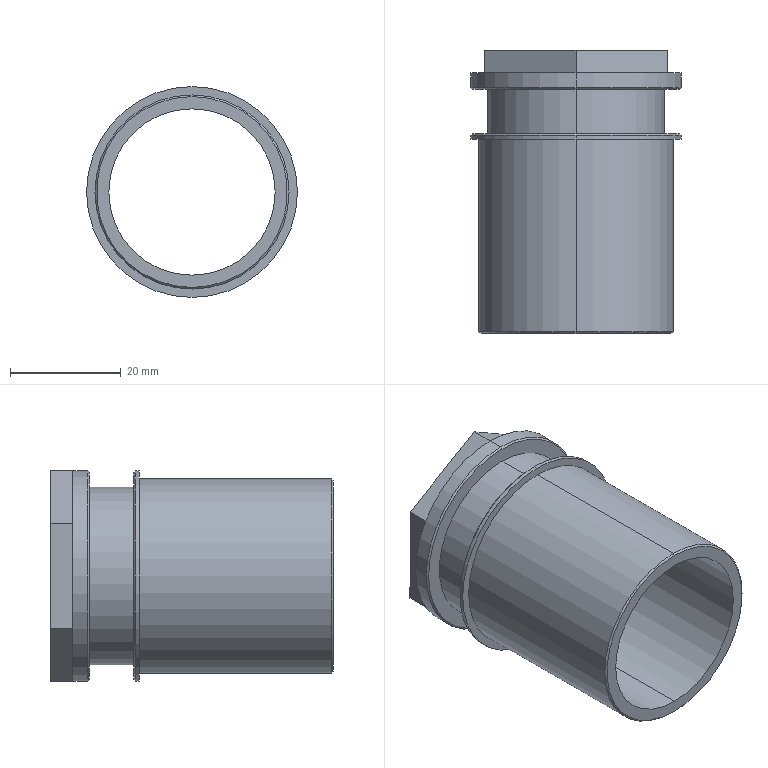Part | SolidWorks | features BaseBody 1 | 1 solid | 33 faces | box 38 x 51 x 38 mm | volume 12331 mm3 | plane 17 | cylinder 10 | cone 6 | commonest cylinder face diameters 38 x4 30 x2 32 x2 35 x2
STEP:
#1=CARTESIAN_POINT('',(0.,0.,-17.2));
#2=VERTEX_POINT('',#1);
#3=CARTESIAN_POINT('',(0.,0.,17.2));
#4=VERTEX_POINT('',#3);
#5=CARTESIAN_POINT('',(0.,0.,0.));
#6=DIRECTION('',(0.,-1.,0.));
#7=DIRECTION('',(0.,0.,1.));
#8=AXIS2_PLACEMENT_3D('',#5,#6,#7);
#9=CIRCLE('',#8,17.2);
#10=EDGE_CURVE('',#2,#4,#9,.T.);
#11=ORIENTED_EDGE('',*,*,#10,.F.);
#12=CARTESIAN_POINT('',(0.,0.3,-17.5));
#13=VERTEX_POINT('',#12);
#14=CARTESIAN_POINT('',(0.,0.3,-17.5));
#15=DIRECTION('',(0.,0.7071,-0.7071));
#16=VECTOR('',#15,1000.);
#17=LINE('',#14,#16);
#18=EDGE_CURVE('',#2,#13,#17,.T.);
#19=ORIENTED_EDGE('',*,*,#18,.T.);
#20=CARTESIAN_POINT('',(0.,0.3,17.5));
#21=VERTEX_POINT('',#20);
#22=CARTESIAN_POINT('',(0.,0.3,0.));
#23=DIRECTION('',(0.,1.,0.));
#24=DIRECTION('',(0.,0.,1.));
#25=AXIS2_PLACEMENT_3D('',#22,#23,#24);
#26=CIRCLE('',#25,17.5);
#27=EDGE_CURVE('',#21,#13,#26,.T.);
#28=ORIENTED_EDGE('',*,*,#27,.F.);
#29=CARTESIAN_POINT('',(0.,0.3,17.5));
#30=DIRECTION('',(0.,0.7071,0.7071));
#31=VECTOR('',#30,1000.);
#32=LINE('',#29,#31);
#33=EDGE_CURVE('',#4,#21,#32,.T.);
#34=ORIENTED_EDGE('',*,*,#33,.F.);
#35=EDGE_LOOP('',(#11,#19,#28,#34));
#36=FACE_OUTER_BOUND('',#35,.T.);
#37=CARTESIAN_POINT('',(0.,0.3,0.));
#38=DIRECTION('',(0.,1.,0.));
#39=DIRECTION('',(0.,0.,1.));
#40=AXIS2_PLACEMENT_3D('',#37,#38,#39);
#41=CONICAL_SURFACE('',#40,17.5,0.7854);
#42=ADVANCED_FACE('',(#36),#41,.T.);
#43=CARTESIAN_POINT('',(0.,44.,-18.7));
#44=VERTEX_POINT('',#43);
#45=CARTESIAN_POINT('',(0.,44.,18.7));
#46=VERTEX_POINT('',#45);
#47=CARTESIAN_POINT('',(0.,44.,0.));
#48=DIRECTION('',(0.,-1.,0.));
#49=DIRECTION('',(0.,0.,1.));
#50=AXIS2_PLACEMENT_3D('',#47,#48,#49);
#51=CIRCLE('',#50,18.7);
#52=EDGE_CURVE('',#44,#46,#51,.T.);
#53=ORIENTED_EDGE('',*,*,#52,.F.);
#54=CARTESIAN_POINT('',(0.,44.3,-19.));
#55=VERTEX_POINT('',#54);
#56=CARTESIAN_POINT('',(0.,44.3,-19.));
#57=DIRECTION('',(0.,0.7071,-0.7071));
#58=VECTOR('',#57,1000.);
#59=LINE('',#56,#58);
#60=EDGE_CURVE('',#44,#55,#59,.T.);
#61=ORIENTED_EDGE('',*,*,#60,.T.);
#62=CARTESIAN_POINT('',(0.,44.3,19.));
#63=VERTEX_POINT('',#62);
#64=CARTESIAN_POINT('',(0.,44.3,0.));
#65=DIRECTION('',(0.,1.,0.));
#66=DIRECTION('',(0.,0.,1.));
#67=AXIS2_PLACEMENT_3D('',#64,#65,#66);
#68=CIRCLE('',#67,19.);
#69=EDGE_CURVE('',#63,#55,#68,.T.);
#70=ORIENTED_EDGE('',*,*,#69,.F.);
#71=CARTESIAN_POINT('',(0.,44.3,19.));
#72=DIRECTION('',(0.,0.7071,0.7071));
#73=VECTOR('',#72,1000.);
#74=LINE('',#71,#73);
#75=EDGE_CURVE('',#46,#63,#74,.T.);
#76=ORIENTED_EDGE('',*,*,#75,.F.);
#77=EDGE_LOOP('',(#53,#61,#70,#76));
#78=FACE_OUTER_BOUND('',#77,.T.);
#79=CARTESIAN_POINT('',(0.,44.3,0.));
#80=DIRECTION('',(0.,1.,0.));
#81=DIRECTION('',(0.,0.,1.));
#82=AXIS2_PLACEMENT_3D('',#79,#80,#81);
#83=CONICAL_SURFACE('',#82,19.,0.7854);
#84=ADVANCED_FACE('',(#78),#83,.T.);
#85=CARTESIAN_POINT('',(0.,36.,18.7));
#86=VERTEX_POINT('',#85);
#87=CARTESIAN_POINT('',(0.,36.,-18.7));
#88=VERTEX_POINT('',#87);
#89=CARTESIAN_POINT('',(0.,36.,0.));
#90=DIRECTION('',(0.,1.,0.));
#91=DIRECTION('',(0.,0.,1.));
#92=AXIS2_PLACEMENT_3D('',#89,#90,#91);
#93=CIRCLE('',#92,18.7);
#94=EDGE_CURVE('',#86,#88,#93,.T.);
#95=ORIENTED_EDGE('',*,*,#94,.F.);
#96=CARTESIAN_POINT('',(0.,35.7,19.));
#97=VERTEX_POINT('',#96);
#98=CARTESIAN_POINT('',(0.,36.,18.7));
#99=DIRECTION('',(0.,-0.7071,0.7071));
#100=VECTOR('',#99,1000.);
#101=LINE('',#98,#100);
#102=EDGE_CURVE('',#86,#97,#101,.T.);
#103=ORIENTED_EDGE('',*,*,#102,.T.);
#104=CARTESIAN_POINT('',(0.,35.7,-19.));
#105=VERTEX_POINT('',#104);
#106=CARTESIAN_POINT('',(0.,35.7,0.));
#107=DIRECTION('',(0.,-1.,0.));
#108=DIRECTION('',(0.,0.,1.));
#109=AXIS2_PLACEMENT_3D('',#106,#107,#108);
#110=CIRCLE('',#109,19.);
#111=EDGE_CURVE('',#105,#97,#110,.T.);
#112=ORIENTED_EDGE('',*,*,#111,.F.);
#113=CARTESIAN_POINT('',(0.,36.,-18.7));
#114=DIRECTION('',(0.,-0.7071,-0.7071));
#115=VECTOR('',#114,1000.);
#116=LINE('',#113,#115);
#117=EDGE_CURVE('',#88,#105,#116,.T.);
#118=ORIENTED_EDGE('',*,*,#117,.F.);
#119=EDGE_LOOP('',(#95,#103,#112,#118));
#120=FACE_OUTER_BOUND('',#119,.T.);
#121=CARTESIAN_POINT('',(0.,36.,0.));
#122=DIRECTION('',(0.,-1.,0.));
#123=DIRECTION('',(0.,0.,-1.));
#124=AXIS2_PLACEMENT_3D('',#121,#122,#123);
#125=CONICAL_SURFACE('',#124,18.7,0.7854);
#126=ADVANCED_FACE('',(#120),#125,.T.);
#127=CARTESIAN_POINT('',(0.,0.,-15.));
#128=VERTEX_POINT('',#127);
#129=CARTESIAN_POINT('',(0.,0.,15.));
#130=VERTEX_POINT('',#129);
#131=CARTESIAN_POINT('',(0.,0.,0.));
#132=DIRECTION('',(0.,1.,0.));
#133=DIRECTION('',(0.,0.,1.));
#134=AXIS2_PLACEMENT_3D('',#131,#132,#133);
#135=CIRCLE('',#134,15.);
#136=EDGE_CURVE('',#128,#130,#135,.T.);
#137=ORIENTED_EDGE('',*,*,#136,.F.);
#138=CARTESIAN_POINT('',(0.,51.,-15.));
#139=VERTEX_POINT('',#138);
#140=CARTESIAN_POINT('',(0.,0.,-15.));
#141=DIRECTION('',(0.,1.,0.));
#142=VECTOR('',#141,1000.);
#143=LINE('',#140,#142);
#144=EDGE_CURVE('',#128,#139,#143,.T.);
#145=ORIENTED_EDGE('',*,*,#144,.T.);
#146=CARTESIAN_POINT('',(0.,51.,15.));
#147=VERTEX_POINT('',#146);
#148=CARTESIAN_POINT('',(0.,51.,0.));
#149=DIRECTION('',(0.,1.,0.));
#150=DIRECTION('',(0.,0.,1.));
#151=AXIS2_PLACEMENT_3D('',#148,#149,#150);
#152=CIRCLE('',#151,15.);
#153=EDGE_CURVE('',#139,#147,#152,.T.);
#154=ORIENTED_EDGE('',*,*,#153,.T.);
#155=CARTESIAN_POINT('',(0.,0.,15.));
#156=DIRECTION('',(0.,1.,0.));
#157=VECTOR('',#156,1000.);
#158=LINE('',#155,#157);
#159=EDGE_CURVE('',#130,#147,#158,.T.);
#160=ORIENTED_EDGE('',*,*,#159,.F.);
#161=EDGE_LOOP('',(#137,#145,#154,#160));
#162=FACE_OUTER_BOUND('',#161,.T.);
#163=CARTESIAN_POINT('',(0.,0.,0.));
#164=DIRECTION('',(0.,1.,0.));
#165=DIRECTION('',(0.,0.,1.));
#166=AXIS2_PLACEMENT_3D('',#163,#164,#165);
#167=CYLINDRICAL_SURFACE('',#166,15.);
#168=ADVANCED_FACE('',(#162),#167,.F.);
#169=CARTESIAN_POINT('',(0.,35.,19.));
#170=VERTEX_POINT('',#169);
#171=CARTESIAN_POINT('',(0.,35.,-19.));
#172=VERTEX_POINT('',#171);
#173=CARTESIAN_POINT('',(0.,35.,0.));
#174=DIRECTION('',(0.,1.,0.));
#175=DIRECTION('',(0.,0.,1.));
#176=AXIS2_PLACEMENT_3D('',#173,#174,#175);
#177=CIRCLE('',#176,19.);
#178=EDGE_CURVE('',#170,#172,#177,.T.);
#179=ORIENTED_EDGE('',*,*,#178,.T.);
#180=CARTESIAN_POINT('',(0.,35.,-19.));
#181=DIRECTION('',(0.,1.,0.));
#182=VECTOR('',#181,1000.);
#183=LINE('',#180,#182);
#184=EDGE_CURVE('',#172,#105,#183,.T.);
#185=ORIENTED_EDGE('',*,*,#184,.T.);
#186=ORIENTED_EDGE('',*,*,#111,.T.);
#187=CARTESIAN_POINT('',(0.,35.,19.));
#188=DIRECTION('',(0.,1.,0.));
#189=VECTOR('',#188,1000.);
#190=LINE('',#187,#189);
#191=EDGE_CURVE('',#170,#97,#190,.T.);
#192=ORIENTED_EDGE('',*,*,#191,.F.);
#193=EDGE_LOOP('',(#179,#185,#186,#192));
#194=FACE_OUTER_BOUND('',#193,.T.);
#195=CARTESIAN_POINT('',(0.,35.,0.));
#196=DIRECTION('',(0.,1.,0.));
#197=DIRECTION('',(0.,0.,1.));
#198=AXIS2_PLACEMENT_3D('',#195,#196,#197);
#199=CYLINDRICAL_SURFACE('',#198,19.);
#200=ADVANCED_FACE('',(#194),#199,.T.);
#201=CARTESIAN_POINT('',(0.,35.,17.5));
#202=VERTEX_POINT('',#201);
#203=CARTESIAN_POINT('',(0.,35.,-17.5));
#204=VERTEX_POINT('',#203);
#205=CARTESIAN_POINT('',(0.,35.,0.));
#206=DIRECTION('',(0.,1.,0.));
#207=DIRECTION('',(0.,0.,1.));
#208=AXIS2_PLACEMENT_3D('',#205,#206,#207);
#209=CIRCLE('',#208,17.5);
#210=EDGE_CURVE('',#202,#204,#209,.T.);
#211=ORIENTED_EDGE('',*,*,#210,.F.);
#212=CARTESIAN_POINT('',(0.,36.,17.5));
#213=DIRECTION('',(0.,-1.,0.));
#214=VECTOR('',#213,1000.);
#215=LINE('',#212,#214);
#216=EDGE_CURVE('',#202,#21,#215,.T.);
#217=ORIENTED_EDGE('',*,*,#216,.T.);
#218=ORIENTED_EDGE('',*,*,#27,.T.);
#219=CARTESIAN_POINT('',(0.,36.,-17.5));
#220=DIRECTION('',(0.,-1.,0.));
#221=VECTOR('',#220,1000.);
#222=LINE('',#219,#221);
#223=EDGE_CURVE('',#204,#13,#222,.T.);
#224=ORIENTED_EDGE('',*,*,#223,.F.);
#225=EDGE_LOOP('',(#211,#217,#218,#224));
#226=FACE_OUTER_BOUND('',#225,.T.);
#227=CARTESIAN_POINT('',(0.,36.,0.));
#228=DIRECTION('',(0.,-1.,0.));
#229=DIRECTION('',(0.,0.,-1.));
#230=AXIS2_PLACEMENT_3D('',#227,#228,#229);
#231=CYLINDRICAL_SURFACE('',#230,17.5);
#232=ADVANCED_FACE('',(#226),#231,.T.);
#233=CARTESIAN_POINT('',(0.,44.,16.));
#234=VERTEX_POINT('',#233);
#235=CARTESIAN_POINT('',(0.,44.,-16.));
#236=VERTEX_POINT('',#235);
#237=CARTESIAN_POINT('',(0.,44.,0.));
#238=DIRECTION('',(0.,1.,0.));
#239=DIRECTION('',(0.,0.,1.));
#240=AXIS2_PLACEMENT_3D('',#237,#238,#239);
#241=CIRCLE('',#240,16.);
#242=EDGE_CURVE('',#234,#236,#241,.T.);
#243=ORIENTED_EDGE('',*,*,#242,.F.);
#244=CARTESIAN_POINT('',(0.,36.,16.));
#245=VERTEX_POINT('',#244);
#246=CARTESIAN_POINT('',(0.,51.,16.));
#247=DIRECTION('',(0.,-1.,0.));
#248=VECTOR('',#247,1000.);
#249=LINE('',#246,#248);
#250=EDGE_CURVE('',#234,#245,#249,.T.);
#251=ORIENTED_EDGE('',*,*,#250,.T.);
#252=CARTESIAN_POINT('',(0.,36.,-16.));
#253=VERTEX_POINT('',#252);
#254=CARTESIAN_POINT('',(0.,36.,0.));
#255=DIRECTION('',(0.,1.,0.));
#256=DIRECTION('',(0.,0.,1.));
#257=AXIS2_PLACEMENT_3D('',#254,#255,#256);
#258=CIRCLE('',#257,16.);
#259=EDGE_CURVE('',#245,#253,#258,.T.);
#260=ORIENTED_EDGE('',*,*,#259,.T.);
#261=CARTESIAN_POINT('',(0.,51.,-16.));
#262=DIRECTION('',(0.,-1.,0.));
#263=VECTOR('',#262,1000.);
#264=LINE('',#261,#263);
#265=EDGE_CURVE('',#236,#253,#264,.T.);
#266=ORIENTED_EDGE('',*,*,#265,.F.);
#267=EDGE_LOOP('',(#243,#251,#260,#266));
#268=FACE_OUTER_BOUND('',#267,.T.);
#269=CARTESIAN_POINT('',(0.,51.,0.));
#270=DIRECTION('',(0.,-1.,0.));
#271=DIRECTION('',(0.,0.,-1.));
#272=AXIS2_PLACEMENT_3D('',#269,#270,#271);
#273=CYLINDRICAL_SURFACE('',#272,16.);
#274=ADVANCED_FACE('',(#268),#273,.T.);
#275=ORIENTED_EDGE('',*,*,#69,.T.);
#276=CARTESIAN_POINT('',(0.,47.,-19.));
#277=VERTEX_POINT('',#276);
#278=CARTESIAN_POINT('',(0.,44.,-19.));
#279=DIRECTION('',(0.,1.,0.));
#280=VECTOR('',#279,1000.);
#281=LINE('',#278,#280);
#282=EDGE_CURVE('',#55,#277,#281,.T.);
#283=ORIENTED_EDGE('',*,*,#282,.T.);
#284=CARTESIAN_POINT('',(16.454,47.,-9.5));
#285=VERTEX_POINT('',#284);
#286=CARTESIAN_POINT('',(0.,47.,0.));
#287=DIRECTION('',(0.,-1.,0.));
#288=DIRECTION('',(0.,0.,1.));
#289=AXIS2_PLACEMENT_3D('',#286,#287,#288);
#290=CIRCLE('',#289,19.);
#291=EDGE_CURVE('',#277,#285,#290,.T.);
#292=ORIENTED_EDGE('',*,*,#291,.T.);
#293=CARTESIAN_POINT('',(16.454,47.,9.5));
#294=VERTEX_POINT('',#293);
#295=CARTESIAN_POINT('',(0.,47.,0.));
#296=DIRECTION('',(0.,-1.,0.));
#297=DIRECTION('',(0.,0.,1.));
#298=AXIS2_PLACEMENT_3D('',#295,#296,#297);
#299=CIRCLE('',#298,19.);
#300=EDGE_CURVE('',#285,#294,#299,.T.);
#301=ORIENTED_EDGE('',*,*,#300,.T.);
#302=CARTESIAN_POINT('',(0.,47.,19.));
#303=VERTEX_POINT('',#302);
#304=CARTESIAN_POINT('',(0.,47.,0.));
#305=DIRECTION('',(0.,-1.,0.));
#306=DIRECTION('',(0.,0.,1.));
#307=AXIS2_PLACEMENT_3D('',#304,#305,#306);
#308=CIRCLE('',#307,19.);
#309=EDGE_CURVE('',#294,#303,#308,.T.);
#310=ORIENTED_EDGE('',*,*,#309,.T.);
#311=CARTESIAN_POINT('',(0.,44.,19.));
#312=DIRECTION('',(0.,1.,0.));
#313=VECTOR('',#312,1000.);
#314=LINE('',#311,#313);
#315=EDGE_CURVE('',#63,#303,#314,.T.);
#316=ORIENTED_EDGE('',*,*,#315,.F.);
#317=EDGE_LOOP('',(#275,#283,#292,#301,#310,#316));
#318=FACE_OUTER_BOUND('',#317,.T.);
#319=CARTESIAN_POINT('',(0.,44.,0.));
#320=DIRECTION('',(0.,1.,0.));
#321=DIRECTION('',(0.,0.,1.));
#322=AXIS2_PLACEMENT_3D('',#319,#320,#321);
#323=CYLINDRICAL_SURFACE('',#322,19.);
#324=ADVANCED_FACE('',(#318),#323,.T.);
#325=CARTESIAN_POINT('',(0.,51.,-19.));
#326=VERTEX_POINT('',#325);
#327=CARTESIAN_POINT('',(-16.454,51.,-9.5));
#328=VERTEX_POINT('',#327);
#329=CARTESIAN_POINT('',(0.,51.,-19.));
#330=DIRECTION('',(-0.866,0.,0.5));
#331=VECTOR('',#330,1000.);
#332=LINE('',#329,#331);
#333=EDGE_CURVE('',#326,#328,#332,.T.);
#334=ORIENTED_EDGE('',*,*,#333,.F.);
#335=CARTESIAN_POINT('',(0.,47.,-19.));
#336=DIRECTION('',(0.,1.,0.));
#337=VECTOR('',#336,1000.);
#338=LINE('',#335,#337);
#339=EDGE_CURVE('',#277,#326,#338,.T.);
#340=ORIENTED_EDGE('',*,*,#339,.F.);
#341=CARTESIAN_POINT('',(-16.454,47.,-9.5));
#342=VERTEX_POINT('',#341);
#343=CARTESIAN_POINT('',(0.,47.,-19.));
#344=DIRECTION('',(-0.866,0.,0.5));
#345=VECTOR('',#344,1000.);
#346=LINE('',#343,#345);
#347=EDGE_CURVE('',#277,#342,#346,.T.);
#348=ORIENTED_EDGE('',*,*,#347,.T.);
#349=CARTESIAN_POINT('',(-16.454,47.,-9.5));
#350=DIRECTION('',(0.,1.,0.));
#351=VECTOR('',#350,1000.);
#352=LINE('',#349,#351);
#353=EDGE_CURVE('',#342,#328,#352,.T.);
#354=ORIENTED_EDGE('',*,*,#353,.T.);
#355=EDGE_LOOP('',(#334,#340,#348,#354));
#356=FACE_OUTER_BOUND('',#355,.T.);
#357=CARTESIAN_POINT('',(0.,47.,-19.));
#358=DIRECTION('',(-0.5,0.,-0.866));
#359=DIRECTION('',(-0.866,0.,0.5));
#360=AXIS2_PLACEMENT_3D('',#357,#358,#359);
#361=PLANE('',#360);
#362=ADVANCED_FACE('',(#356),#361,.T.);
#363=CARTESIAN_POINT('',(-16.454,51.,9.5));
#364=VERTEX_POINT('',#363);
#365=CARTESIAN_POINT('',(-16.454,51.,-9.5));
#366=DIRECTION('',(0.,0.,1.));
#367=VECTOR('',#366,1000.);
#368=LINE('',#365,#367);
#369=EDGE_CURVE('',#328,#364,#368,.T.);
#370=ORIENTED_EDGE('',*,*,#369,.F.);
#371=ORIENTED_EDGE('',*,*,#353,.F.);
#372=CARTESIAN_POINT('',(-16.454,47.,9.5));
#373=VERTEX_POINT('',#372);
#374=CARTESIAN_POINT('',(-16.454,47.,-9.5));
#375=DIRECTION('',(0.,0.,1.));
#376=VECTOR('',#375,1000.);
#377=LINE('',#374,#376);
#378=EDGE_CURVE('',#342,#373,#377,.T.);
#379=ORIENTED_EDGE('',*,*,#378,.T.);
#380=CARTESIAN_POINT('',(-16.454,47.,9.5));
#381=DIRECTION('',(0.,1.,0.));
#382=VECTOR('',#381,1000.);
#383=LINE('',#380,#382);
#384=EDGE_CURVE('',#373,#364,#383,.T.);
#385=ORIENTED_EDGE('',*,*,#384,.T.);
#386=EDGE_LOOP('',(#370,#371,#379,#385));
#387=FACE_OUTER_BOUND('',#386,.T.);
#388=CARTESIAN_POINT('',(-16.454,47.,-9.5));
#389=DIRECTION('',(-1.,0.,0.));
#390=DIRECTION('',(0.,1.,0.));
#391=AXIS2_PLACEMENT_3D('',#388,#389,#390);
#392=PLANE('',#391);
#393=ADVANCED_FACE('',(#387),#392,.T.);
#394=CARTESIAN_POINT('',(0.,51.,19.));
#395=VERTEX_POINT('',#394);
#396=CARTESIAN_POINT('',(-16.454,51.,9.5));
#397=DIRECTION('',(0.866,0.,0.5));
#398=VECTOR('',#397,1000.);
#399=LINE('',#396,#398);
#400=EDGE_CURVE('',#364,#395,#399,.T.);
#401=ORIENTED_EDGE('',*,*,#400,.F.);
#402=ORIENTED_EDGE('',*,*,#384,.F.);
#403=CARTESIAN_POINT('',(-16.454,47.,9.5));
#404=DIRECTION('',(0.866,0.,0.5));
#405=VECTOR('',#404,1000.);
#406=LINE('',#403,#405);
#407=EDGE_CURVE('',#373,#303,#406,.T.);
#408=ORIENTED_EDGE('',*,*,#407,.T.);
#409=CARTESIAN_POINT('',(0.,47.,19.));
#410=DIRECTION('',(0.,1.,0.));
#411=VECTOR('',#410,1000.);
#412=LINE('',#409,#411);
#413=EDGE_CURVE('',#303,#395,#412,.T.);
#414=ORIENTED_EDGE('',*,*,#413,.T.);
#415=EDGE_LOOP('',(#401,#402,#408,#414));
#416=FACE_OUTER_BOUND('',#415,.T.);
#417=CARTESIAN_POINT('',(-16.454,47.,9.5));
#418=DIRECTION('',(-0.5,0.,0.866));
#419=DIRECTION('',(0.,1.,0.));
#420=AXIS2_PLACEMENT_3D('',#417,#418,#419);
#421=PLANE('',#420);
#422=ADVANCED_FACE('',(#416),#421,.T.);
#423=CARTESIAN_POINT('',(16.454,51.,9.5));
#424=VERTEX_POINT('',#423);
#425=CARTESIAN_POINT('',(0.,51.,19.));
#426=DIRECTION('',(0.866,0.,-0.5));
#427=VECTOR('',#426,1000.);
#428=LINE('',#425,#427);
#429=EDGE_CURVE('',#395,#424,#428,.T.);
#430=ORIENTED_EDGE('',*,*,#429,.F.);
#431=ORIENTED_EDGE('',*,*,#413,.F.);
#432=CARTESIAN_POINT('',(0.,47.,19.));
#433=DIRECTION('',(0.866,0.,-0.5));
#434=VECTOR('',#433,1000.);
#435=LINE('',#432,#434);
#436=EDGE_CURVE('',#303,#294,#435,.T.);
#437=ORIENTED_EDGE('',*,*,#436,.T.);
#438=CARTESIAN_POINT('',(16.454,47.,9.5));
#439=DIRECTION('',(0.,1.,0.));
#440=VECTOR('',#439,1000.);
#441=LINE('',#438,#440);
#442=EDGE_CURVE('',#294,#424,#441,.T.);
#443=ORIENTED_EDGE('',*,*,#442,.T.);
#444=EDGE_LOOP('',(#430,#431,#437,#443));
#445=FACE_OUTER_BOUND('',#444,.T.);
#446=CARTESIAN_POINT('',(0.,47.,19.));
#447=DIRECTION('',(0.5,0.,0.866));
#448=DIRECTION('',(0.,-1.,0.));
#449=AXIS2_PLACEMENT_3D('',#446,#447,#448);
#450=PLANE('',#449);
#451=ADVANCED_FACE('',(#445),#450,.T.);
#452=CARTESIAN_POINT('',(16.454,51.,-9.5));
#453=VERTEX_POINT('',#452);
#454=CARTESIAN_POINT('',(16.454,51.,9.5));
#455=DIRECTION('',(0.,0.,-1.));
#456=VECTOR('',#455,1000.);
#457=LINE('',#454,#456);
#458=EDGE_CURVE('',#424,#453,#457,.T.);
#459=ORIENTED_EDGE('',*,*,#458,.F.);
#460=ORIENTED_EDGE('',*,*,#442,.F.);
#461=CARTESIAN_POINT('',(16.454,47.,9.5));
#462=DIRECTION('',(0.,0.,-1.));
#463=VECTOR('',#462,1000.);
#464=LINE('',#461,#463);
#465=EDGE_CURVE('',#294,#285,#464,.T.);
#466=ORIENTED_EDGE('',*,*,#465,.T.);
#467=CARTESIAN_POINT('',(16.454,47.,-9.5));
#468=DIRECTION('',(0.,1.,0.));
#469=VECTOR('',#468,1000.);
#470=LINE('',#467,#469);
#471=EDGE_CURVE('',#285,#453,#470,.T.);
#472=ORIENTED_EDGE('',*,*,#471,.T.);
#473=EDGE_LOOP('',(#459,#460,#466,#472));
#474=FACE_OUTER_BOUND('',#473,.T.);
#475=CARTESIAN_POINT('',(16.454,47.,9.5));
#476=DIRECTION('',(1.,0.,0.));
#477=DIRECTION('',(0.,1.,0.));
#478=AXIS2_PLACEMENT_3D('',#475,#476,#477);
#479=PLANE('',#478);
#480=ADVANCED_FACE('',(#474),#479,.T.);
#481=CARTESIAN_POINT('',(16.454,51.,-9.5));
#482=DIRECTION('',(-0.866,0.,-0.5));
#483=VECTOR('',#482,1000.);
#484=LINE('',#481,#483);
#485=EDGE_CURVE('',#453,#326,#484,.T.);
#486=ORIENTED_EDGE('',*,*,#485,.F.);
#487=ORIENTED_EDGE('',*,*,#471,.F.);
#488=CARTESIAN_POINT('',(16.454,47.,-9.5));
#489=DIRECTION('',(-0.866,0.,-0.5));
#490=VECTOR('',#489,1000.);
#491=LINE('',#488,#490);
#492=EDGE_CURVE('',#285,#277,#491,.T.);
#493=ORIENTED_EDGE('',*,*,#492,.T.);
#494=ORIENTED_EDGE('',*,*,#339,.T.);
#495=EDGE_LOOP('',(#486,#487,#493,#494));
#496=FACE_OUTER_BOUND('',#495,.T.);
#497=CARTESIAN_POINT('',(16.454,47.,-9.5));
#498=DIRECTION('',(0.5,0.,-0.866));
#499=DIRECTION('',(0.,-1.,0.));
#500=AXIS2_PLACEMENT_3D('',#497,#498,#499);
#501=PLANE('',#500);
#502=ADVANCED_FACE('',(#496),#501,.T.);
#503=ORIENTED_EDGE('',*,*,#436,.F.);
#504=ORIENTED_EDGE('',*,*,#309,.F.);
#505=EDGE_LOOP('',(#503,#504));
#506=FACE_OUTER_BOUND('',#505,.T.);
#507=CARTESIAN_POINT('',(0.,47.,0.));
#508=DIRECTION('',(0.,1.,0.));
#509=DIRECTION('',(1.,0.,0.));
#510=AXIS2_PLACEMENT_3D('',#507,#508,#509);
#511=PLANE('',#510);
#512=ADVANCED_FACE('',(#506),#511,.T.);
#513=ORIENTED_EDGE('',*,*,#465,.F.);
#514=ORIENTED_EDGE('',*,*,#300,.F.);
#515=EDGE_LOOP('',(#513,#514));
#516=FACE_OUTER_BOUND('',#515,.T.);
#517=CARTESIAN_POINT('',(0.,47.,0.));
#518=DIRECTION('',(0.,1.,0.));
#519=DIRECTION('',(1.,0.,0.));
#520=AXIS2_PLACEMENT_3D('',#517,#518,#519);
#521=PLANE('',#520);
#522=ADVANCED_FACE('',(#516),#521,.T.);
#523=ORIENTED_EDGE('',*,*,#492,.F.);
#524=ORIENTED_EDGE('',*,*,#291,.F.);
#525=EDGE_LOOP('',(#523,#524));
#526=FACE_OUTER_BOUND('',#525,.T.);
#527=CARTESIAN_POINT('',(0.,47.,0.));
#528=DIRECTION('',(0.,1.,0.));
#529=DIRECTION('',(1.,0.,0.));
#530=AXIS2_PLACEMENT_3D('',#527,#528,#529);
#531=PLANE('',#530);
#532=ADVANCED_FACE('',(#526),#531,.T.);
#533=ORIENTED_EDGE('',*,*,#347,.F.);
#534=CARTESIAN_POINT('',(0.,47.,0.));
#535=DIRECTION('',(0.,-1.,0.));
#536=DIRECTION('',(0.,0.,1.));
#537=AXIS2_PLACEMENT_3D('',#534,#535,#536);
#538=CIRCLE('',#537,19.);
#539=EDGE_CURVE('',#342,#277,#538,.T.);
#540=ORIENTED_EDGE('',*,*,#539,.F.);
#541=EDGE_LOOP('',(#533,#540));
#542=FACE_OUTER_BOUND('',#541,.T.);
#543=CARTESIAN_POINT('',(0.,47.,0.));
#544=DIRECTION('',(0.,1.,0.));
#545=DIRECTION('',(1.,0.,0.));
#546=AXIS2_PLACEMENT_3D('',#543,#544,#545);
#547=PLANE('',#546);
#548=ADVANCED_FACE('',(#542),#547,.T.);
#549=ORIENTED_EDGE('',*,*,#378,.F.);
#550=CARTESIAN_POINT('',(0.,47.,0.));
#551=DIRECTION('',(0.,-1.,0.));
#552=DIRECTION('',(0.,0.,1.));
#553=AXIS2_PLACEMENT_3D('',#550,#551,#552);
#554=CIRCLE('',#553,19.);
#555=EDGE_CURVE('',#373,#342,#554,.T.);
#556=ORIENTED_EDGE('',*,*,#555,.F.);
#557=EDGE_LOOP('',(#549,#556));
#558=FACE_OUTER_BOUND('',#557,.T.);
#559=CARTESIAN_POINT('',(0.,47.,0.));
#560=DIRECTION('',(0.,1.,0.));
#561=DIRECTION('',(1.,0.,0.));
#562=AXIS2_PLACEMENT_3D('',#559,#560,#561);
#563=PLANE('',#562);
#564=ADVANCED_FACE('',(#558),#563,.T.);
#565=ORIENTED_EDGE('',*,*,#407,.F.);
#566=CARTESIAN_POINT('',(0.,47.,0.));
#567=DIRECTION('',(0.,-1.,0.));
#568=DIRECTION('',(0.,0.,1.));
#569=AXIS2_PLACEMENT_3D('',#566,#567,#568);
#570=CIRCLE('',#569,19.);
#571=EDGE_CURVE('',#303,#373,#570,.T.);
#572=ORIENTED_EDGE('',*,*,#571,.F.);
#573=EDGE_LOOP('',(#565,#572));
#574=FACE_OUTER_BOUND('',#573,.T.);
#575=CARTESIAN_POINT('',(0.,47.,0.));
#576=DIRECTION('',(0.,1.,0.));
#577=DIRECTION('',(1.,0.,0.));
#578=AXIS2_PLACEMENT_3D('',#575,#576,#577);
#579=PLANE('',#578);
#580=ADVANCED_FACE('',(#574),#579,.T.);
#581=CARTESIAN_POINT('',(0.,44.,0.));
#582=DIRECTION('',(0.,1.,0.));
#583=DIRECTION('',(0.,0.,1.));
#584=AXIS2_PLACEMENT_3D('',#581,#582,#583);
#585=CIRCLE('',#584,16.);
#586=EDGE_CURVE('',#236,#234,#585,.T.);
#587=ORIENTED_EDGE('',*,*,#586,.T.);
#588=ORIENTED_EDGE('',*,*,#242,.T.);
#589=EDGE_LOOP('',(#587,#588));
#590=FACE_BOUND('',#589,.T.);
#591=CARTESIAN_POINT('',(0.,44.,0.));
#592=DIRECTION('',(0.,-1.,0.));
#593=DIRECTION('',(0.,0.,1.));
#594=AXIS2_PLACEMENT_3D('',#591,#592,#593);
#595=CIRCLE('',#594,18.7);
#596=EDGE_CURVE('',#46,#44,#595,.T.);
#597=ORIENTED_EDGE('',*,*,#596,.T.);
#598=ORIENTED_EDGE('',*,*,#52,.T.);
#599=EDGE_LOOP('',(#597,#598));
#600=FACE_OUTER_BOUND('',#599,.T.);
#601=CARTESIAN_POINT('',(0.,44.,0.));
#602=DIRECTION('',(0.,1.,0.));
#603=DIRECTION('',(1.,0.,0.));
#604=AXIS2_PLACEMENT_3D('',#601,#602,#603);
#605=PLANE('',#604);
#606=ADVANCED_FACE('',(#590,#600),#605,.F.);
#607=CARTESIAN_POINT('',(0.,36.,0.));
#608=DIRECTION('',(0.,1.,0.));
#609=DIRECTION('',(0.,0.,1.));
#610=AXIS2_PLACEMENT_3D('',#607,#608,#609);
#611=CIRCLE('',#610,16.);
#612=EDGE_CURVE('',#253,#245,#611,.T.);
#613=ORIENTED_EDGE('',*,*,#612,.F.);
#614=ORIENTED_EDGE('',*,*,#259,.F.);
#615=EDGE_LOOP('',(#613,#614));
#616=FACE_BOUND('',#615,.T.);
#617=CARTESIAN_POINT('',(0.,36.,0.));
#618=DIRECTION('',(0.,1.,0.));
#619=DIRECTION('',(0.,0.,1.));
#620=AXIS2_PLACEMENT_3D('',#617,#618,#619);
#621=CIRCLE('',#620,18.7);
#622=EDGE_CURVE('',#88,#86,#621,.T.);
#623=ORIENTED_EDGE('',*,*,#622,.T.);
#624=ORIENTED_EDGE('',*,*,#94,.T.);
#625=EDGE_LOOP('',(#623,#624));
#626=FACE_OUTER_BOUND('',#625,.T.);
#627=CARTESIAN_POINT('',(0.,36.,0.));
#628=DIRECTION('',(0.,1.,0.));
#629=DIRECTION('',(1.,0.,0.));
#630=AXIS2_PLACEMENT_3D('',#627,#628,#629);
#631=PLANE('',#630);
#632=ADVANCED_FACE('',(#616,#626),#631,.T.);
#633=CARTESIAN_POINT('',(0.,35.,0.));
#634=DIRECTION('',(0.,1.,0.));
#635=DIRECTION('',(0.,0.,1.));
#636=AXIS2_PLACEMENT_3D('',#633,#634,#635);
#637=CIRCLE('',#636,17.5);
#638=EDGE_CURVE('',#204,#202,#637,.T.);
#639=ORIENTED_EDGE('',*,*,#638,.T.);
#640=ORIENTED_EDGE('',*,*,#210,.T.);
#641=EDGE_LOOP('',(#639,#640));
#642=FACE_BOUND('',#641,.T.);
#643=ORIENTED_EDGE('',*,*,#178,.F.);
#644=CARTESIAN_POINT('',(0.,35.,0.));
#645=DIRECTION('',(0.,1.,0.));
#646=DIRECTION('',(0.,0.,1.));
#647=AXIS2_PLACEMENT_3D('',#644,#645,#646);
#648=CIRCLE('',#647,19.);
#649=EDGE_CURVE('',#172,#170,#648,.T.);
#650=ORIENTED_EDGE('',*,*,#649,.F.);
#651=EDGE_LOOP('',(#643,#650));
#652=FACE_OUTER_BOUND('',#651,.T.);
#653=CARTESIAN_POINT('',(0.,35.,0.));
#654=DIRECTION('',(0.,1.,0.));
#655=DIRECTION('',(1.,0.,0.));
#656=AXIS2_PLACEMENT_3D('',#653,#654,#655);
#657=PLANE('',#656);
#658=ADVANCED_FACE('',(#642,#652),#657,.F.);
#659=CARTESIAN_POINT('',(0.,0.,0.));
#660=DIRECTION('',(0.,1.,0.));
#661=DIRECTION('',(0.,0.,1.));
#662=AXIS2_PLACEMENT_3D('',#659,#660,#661);
#663=CIRCLE('',#662,15.);
#664=EDGE_CURVE('',#130,#128,#663,.T.);
#665=ORIENTED_EDGE('',*,*,#664,.T.);
#666=ORIENTED_EDGE('',*,*,#136,.T.);
#667=EDGE_LOOP('',(#665,#666));
#668=FACE_BOUND('',#667,.T.);
#669=CARTESIAN_POINT('',(0.,0.,0.));
#670=DIRECTION('',(0.,-1.,0.));
#671=DIRECTION('',(0.,0.,1.));
#672=AXIS2_PLACEMENT_3D('',#669,#670,#671);
#673=CIRCLE('',#672,17.2);
#674=EDGE_CURVE('',#4,#2,#673,.T.);
#675=ORIENTED_EDGE('',*,*,#674,.T.);
#676=ORIENTED_EDGE('',*,*,#10,.T.);
#677=EDGE_LOOP('',(#675,#676));
#678=FACE_OUTER_BOUND('',#677,.T.);
#679=CARTESIAN_POINT('',(0.,0.,0.));
#680=DIRECTION('',(0.,1.,0.));
#681=DIRECTION('',(1.,0.,0.));
#682=AXIS2_PLACEMENT_3D('',#679,#680,#681);
#683=PLANE('',#682);
#684=ADVANCED_FACE('',(#668,#678),#683,.F.);
#685=CARTESIAN_POINT('',(0.,51.,0.));
#686=DIRECTION('',(0.,1.,0.));
#687=DIRECTION('',(0.,0.,1.));
#688=AXIS2_PLACEMENT_3D('',#685,#686,#687);
#689=CIRCLE('',#688,15.);
#690=EDGE_CURVE('',#147,#139,#689,.T.);
#691=ORIENTED_EDGE('',*,*,#690,.F.);
#692=ORIENTED_EDGE('',*,*,#153,.F.);
#693=EDGE_LOOP('',(#691,#692));
#694=FACE_BOUND('',#693,.T.);
#695=ORIENTED_EDGE('',*,*,#458,.T.);
#696=ORIENTED_EDGE('',*,*,#485,.T.);
#697=ORIENTED_EDGE('',*,*,#333,.T.);
#698=ORIENTED_EDGE('',*,*,#369,.T.);
#699=ORIENTED_EDGE('',*,*,#400,.T.);
#700=ORIENTED_EDGE('',*,*,#429,.T.);
#701=EDGE_LOOP('',(#695,#696,#697,#698,#699,#700));
#702=FACE_OUTER_BOUND('',#701,.T.);
#703=CARTESIAN_POINT('',(0.,51.,0.));
#704=DIRECTION('',(0.,1.,0.));
#705=DIRECTION('',(1.,0.,0.));
#706=AXIS2_PLACEMENT_3D('',#703,#704,#705);
#707=PLANE('',#706);
#708=ADVANCED_FACE('',(#694,#702),#707,.T.);
#709=ORIENTED_EDGE('',*,*,#282,.F.);
#710=CARTESIAN_POINT('',(0.,44.3,0.));
#711=DIRECTION('',(0.,1.,0.));
#712=DIRECTION('',(0.,0.,1.));
#713=AXIS2_PLACEMENT_3D('',#710,#711,#712);
#714=CIRCLE('',#713,19.);
#715=EDGE_CURVE('',#55,#63,#714,.T.);
#716=ORIENTED_EDGE('',*,*,#715,.T.);
#717=ORIENTED_EDGE('',*,*,#315,.T.);
#718=ORIENTED_EDGE('',*,*,#571,.T.);
#719=ORIENTED_EDGE('',*,*,#555,.T.);
#720=ORIENTED_EDGE('',*,*,#539,.T.);
#721=EDGE_LOOP('',(#709,#716,#717,#718,#719,#720));
#722=FACE_OUTER_BOUND('',#721,.T.);
#723=CARTESIAN_POINT('',(0.,44.,0.));
#724=DIRECTION('',(0.,1.,0.));
#725=DIRECTION('',(0.,0.,1.));
#726=AXIS2_PLACEMENT_3D('',#723,#724,#725);
#727=CYLINDRICAL_SURFACE('',#726,19.);
#728=ADVANCED_FACE('',(#722),#727,.T.);
#729=ORIENTED_EDGE('',*,*,#250,.F.);
#730=ORIENTED_EDGE('',*,*,#586,.F.);
#731=ORIENTED_EDGE('',*,*,#265,.T.);
#732=ORIENTED_EDGE('',*,*,#612,.T.);
#733=EDGE_LOOP('',(#729,#730,#731,#732));
#734=FACE_OUTER_BOUND('',#733,.T.);
#735=CARTESIAN_POINT('',(0.,51.,0.));
#736=DIRECTION('',(0.,-1.,0.));
#737=DIRECTION('',(0.,0.,-1.));
#738=AXIS2_PLACEMENT_3D('',#735,#736,#737);
#739=CYLINDRICAL_SURFACE('',#738,16.);
#740=ADVANCED_FACE('',(#734),#739,.T.);
#741=ORIENTED_EDGE('',*,*,#216,.F.);
#742=ORIENTED_EDGE('',*,*,#638,.F.);
#743=ORIENTED_EDGE('',*,*,#223,.T.);
#744=CARTESIAN_POINT('',(0.,0.3,0.));
#745=DIRECTION('',(0.,1.,0.));
#746=DIRECTION('',(0.,0.,1.));
#747=AXIS2_PLACEMENT_3D('',#744,#745,#746);
#748=CIRCLE('',#747,17.5);
#749=EDGE_CURVE('',#13,#21,#748,.T.);
#750=ORIENTED_EDGE('',*,*,#749,.T.);
#751=EDGE_LOOP('',(#741,#742,#743,#750));
#752=FACE_OUTER_BOUND('',#751,.T.);
#753=CARTESIAN_POINT('',(0.,36.,0.));
#754=DIRECTION('',(0.,-1.,0.));
#755=DIRECTION('',(0.,0.,-1.));
#756=AXIS2_PLACEMENT_3D('',#753,#754,#755);
#757=CYLINDRICAL_SURFACE('',#756,17.5);
#758=ADVANCED_FACE('',(#752),#757,.T.);
#759=ORIENTED_EDGE('',*,*,#184,.F.);
#760=ORIENTED_EDGE('',*,*,#649,.T.);
#761=ORIENTED_EDGE('',*,*,#191,.T.);
#762=CARTESIAN_POINT('',(0.,35.7,0.));
#763=DIRECTION('',(0.,-1.,0.));
#764=DIRECTION('',(0.,0.,1.));
#765=AXIS2_PLACEMENT_3D('',#762,#763,#764);
#766=CIRCLE('',#765,19.);
#767=EDGE_CURVE('',#97,#105,#766,.T.);
#768=ORIENTED_EDGE('',*,*,#767,.T.);
#769=EDGE_LOOP('',(#759,#760,#761,#768));
#770=FACE_OUTER_BOUND('',#769,.T.);
#771=CARTESIAN_POINT('',(0.,35.,0.));
#772=DIRECTION('',(0.,1.,0.));
#773=DIRECTION('',(0.,0.,1.));
#774=AXIS2_PLACEMENT_3D('',#771,#772,#773);
#775=CYLINDRICAL_SURFACE('',#774,19.);
#776=ADVANCED_FACE('',(#770),#775,.T.);
#777=ORIENTED_EDGE('',*,*,#144,.F.);
#778=ORIENTED_EDGE('',*,*,#664,.F.);
#779=ORIENTED_EDGE('',*,*,#159,.T.);
#780=ORIENTED_EDGE('',*,*,#690,.T.);
#781=EDGE_LOOP('',(#777,#778,#779,#780));
#782=FACE_OUTER_BOUND('',#781,.T.);
#783=CARTESIAN_POINT('',(0.,0.,0.));
#784=DIRECTION('',(0.,1.,0.));
#785=DIRECTION('',(0.,0.,1.));
#786=AXIS2_PLACEMENT_3D('',#783,#784,#785);
#787=CYLINDRICAL_SURFACE('',#786,15.);
#788=ADVANCED_FACE('',(#782),#787,.F.);
#789=ORIENTED_EDGE('',*,*,#102,.F.);
#790=ORIENTED_EDGE('',*,*,#622,.F.);
#791=ORIENTED_EDGE('',*,*,#117,.T.);
#792=ORIENTED_EDGE('',*,*,#767,.F.);
#793=EDGE_LOOP('',(#789,#790,#791,#792));
#794=FACE_OUTER_BOUND('',#793,.T.);
#795=CARTESIAN_POINT('',(0.,36.,0.));
#796=DIRECTION('',(0.,-1.,0.));
#797=DIRECTION('',(0.,0.,-1.));
#798=AXIS2_PLACEMENT_3D('',#795,#796,#797);
#799=CONICAL_SURFACE('',#798,18.7,0.7854);
#800=ADVANCED_FACE('',(#794),#799,.T.);
#801=ORIENTED_EDGE('',*,*,#60,.F.);
#802=ORIENTED_EDGE('',*,*,#596,.F.);
#803=ORIENTED_EDGE('',*,*,#75,.T.);
#804=ORIENTED_EDGE('',*,*,#715,.F.);
#805=EDGE_LOOP('',(#801,#802,#803,#804));
#806=FACE_OUTER_BOUND('',#805,.T.);
#807=CARTESIAN_POINT('',(0.,44.3,0.));
#808=DIRECTION('',(0.,1.,0.));
#809=DIRECTION('',(0.,0.,1.));
#810=AXIS2_PLACEMENT_3D('',#807,#808,#809);
#811=CONICAL_SURFACE('',#810,19.,0.7854);
#812=ADVANCED_FACE('',(#806),#811,.T.);
#813=ORIENTED_EDGE('',*,*,#18,.F.);
#814=ORIENTED_EDGE('',*,*,#674,.F.);
#815=ORIENTED_EDGE('',*,*,#33,.T.);
#816=ORIENTED_EDGE('',*,*,#749,.F.);
#817=EDGE_LOOP('',(#813,#814,#815,#816));
#818=FACE_OUTER_BOUND('',#817,.T.);
#819=CARTESIAN_POINT('',(0.,0.3,0.));
#820=DIRECTION('',(0.,1.,0.));
#821=DIRECTION('',(0.,0.,1.));
#822=AXIS2_PLACEMENT_3D('',#819,#820,#821);
#823=CONICAL_SURFACE('',#822,17.5,0.7854);
#824=ADVANCED_FACE('',(#818),#823,.T.);
#825=CLOSED_SHELL('',(#42,#84,#126,#168,#200,#232,#274,#324,#362,#393,#422,#451,#480,#502,#512,#522,#532,#548,#564,#580,#606,#632,#658,#684,#708,#728,#740,#758,#776,#788,#800,#812,#824));
#826=MANIFOLD_SOLID_BREP('',#825);
#827=CARTESIAN_POINT('',(0.,0.,0.));
#828=DIRECTION('',(0.,0.,1.));
#829=DIRECTION('',(1.,0.,0.));
#830=AXIS2_PLACEMENT_3D('',#827,#828,#829);
#831=(LENGTH_UNIT()NAMED_UNIT(*)SI_UNIT(.MILLI.,.METRE.));
#832=UNCERTAINTY_MEASURE_WITH_UNIT(LENGTH_MEASURE(0.00001),#831,'','');
#833=(NAMED_UNIT(*)PLANE_ANGLE_UNIT()SI_UNIT($,.RADIAN.));
#834=(NAMED_UNIT(*)SI_UNIT($,.STERADIAN.)SOLID_ANGLE_UNIT());
#835=(GEOMETRIC_REPRESENTATION_CONTEXT(3)GLOBAL_UNCERTAINTY_ASSIGNED_CONTEXT((#832))GLOBAL_UNIT_ASSIGNED_CONTEXT((#831,#833,#834))REPRESENTATION_CONTEXT('',''));
#836=ADVANCED_BREP_SHAPE_REPRESENTATION('',(#826,#830),#835);